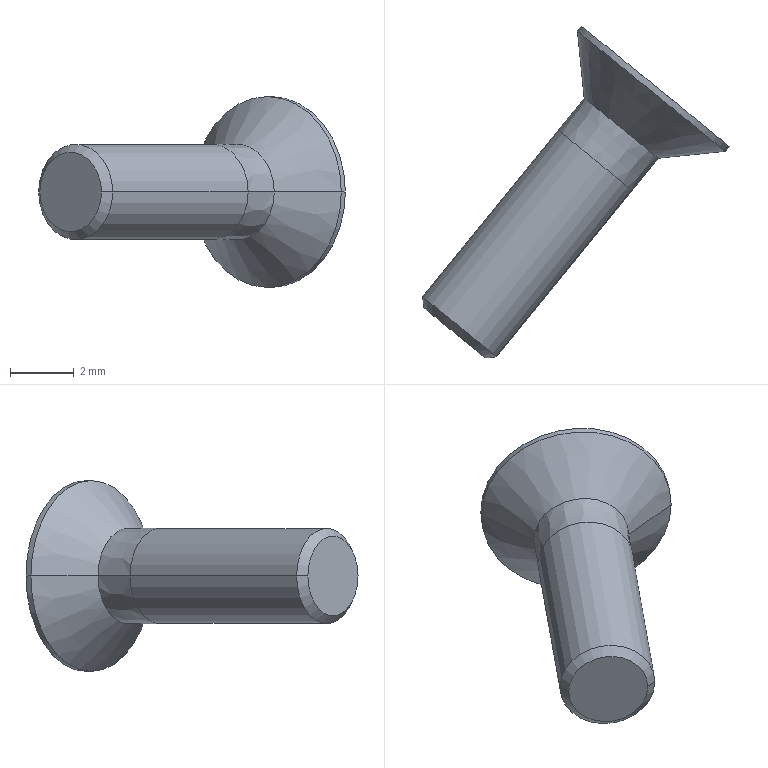Part | SolidWorks | features BaseBody 1 | 1 solid | 20 faces | box 9.643 x 10.44 x 6 mm | volume 84.627 mm3 | plane 10 | cone 6 | cylinder 4 | commonest cylinder face diameters 3 x2 6 x2
STEP:
#1=CARTESIAN_POINT('',(539.658,-134.219,294.945));
#2=VERTEX_POINT('',#1);
#3=CARTESIAN_POINT('',(537.331,-132.326,294.945));
#4=VERTEX_POINT('',#3);
#5=CARTESIAN_POINT('',(538.494,-133.273,294.945));
#6=DIRECTION('',(-0.6309,-0.7758,0.000000012));
#7=DIRECTION('',(0.7758,-0.6309,0.));
#8=AXIS2_PLACEMENT_3D('',#5,#6,#7);
#9=CIRCLE('',#8,1.5);
#10=EDGE_CURVE('',#2,#4,#9,.T.);
#11=ORIENTED_EDGE('',*,*,#10,.T.);
#12=CARTESIAN_POINT('',(533.072,-137.563,294.945));
#13=VERTEX_POINT('',#12);
#14=CARTESIAN_POINT('',(535.201,-134.945,294.945));
#15=DIRECTION('',(-0.6309,-0.7758,0.000000012));
#16=VECTOR('',#15,1000.);
#17=LINE('',#14,#16);
#18=EDGE_CURVE('',#4,#13,#17,.T.);
#19=ORIENTED_EDGE('',*,*,#18,.T.);
#20=CARTESIAN_POINT('',(535.399,-139.456,294.945));
#21=VERTEX_POINT('',#20);
#22=CARTESIAN_POINT('',(534.236,-138.51,294.945));
#23=DIRECTION('',(0.6309,0.7758,-0.000000012));
#24=DIRECTION('',(0.7758,-0.6309,0.));
#25=AXIS2_PLACEMENT_3D('',#22,#23,#24);
#26=CIRCLE('',#25,1.5);
#27=EDGE_CURVE('',#13,#21,#26,.T.);
#28=ORIENTED_EDGE('',*,*,#27,.T.);
#29=CARTESIAN_POINT('',(537.529,-136.838,294.945));
#30=DIRECTION('',(-0.6309,-0.7758,0.000000012));
#31=VECTOR('',#30,1000.);
#32=LINE('',#29,#31);
#33=EDGE_CURVE('',#2,#21,#32,.T.);
#34=ORIENTED_EDGE('',*,*,#33,.F.);
#35=EDGE_LOOP('',(#11,#19,#28,#34));
#36=FACE_OUTER_BOUND('',#35,.T.);
#37=CARTESIAN_POINT('',(536.365,-135.891,294.945));
#38=DIRECTION('',(-0.6309,-0.7758,0.000000012));
#39=DIRECTION('',(0.7758,-0.6309,0.));
#40=AXIS2_PLACEMENT_3D('',#37,#38,#39);
#41=CYLINDRICAL_SURFACE('',#40,1.5);
#42=ADVANCED_FACE('',(#36),#41,.T.);
#43=CARTESIAN_POINT('',(539.443,-132.368,296.435));
#44=VERTEX_POINT('',#43);
#45=CARTESIAN_POINT('',(538.151,-131.318,294.945));
#46=VERTEX_POINT('',#45);
#47=CARTESIAN_POINT('',(539.314,-132.264,294.945));
#48=DIRECTION('',(-0.6309,-0.7758,0.000000012));
#49=DIRECTION('',(0.7758,-0.6309,0.));
#50=AXIS2_PLACEMENT_3D('',#47,#48,#49);
#51=CIRCLE('',#50,1.5);
#52=EDGE_CURVE('',#44,#46,#51,.T.);
#53=ORIENTED_EDGE('',*,*,#52,.T.);
#54=CARTESIAN_POINT('',(537.331,-132.326,294.945));
#55=DIRECTION('',(-0.6311,-0.7757,0.000000012));
#56=VECTOR('',#55,1000.);
#57=LINE('',#54,#56);
#58=EDGE_CURVE('',#46,#4,#57,.T.);
#59=ORIENTED_EDGE('',*,*,#58,.T.);
#60=ORIENTED_EDGE('',*,*,#10,.F.);
#61=CARTESIAN_POINT('',(540.478,-133.21,294.945));
#62=VERTEX_POINT('',#61);
#63=CARTESIAN_POINT('',(539.658,-134.219,294.945));
#64=DIRECTION('',(-0.6307,-0.776,0.000000012));
#65=VECTOR('',#64,1000.);
#66=LINE('',#63,#65);
#67=EDGE_CURVE('',#62,#2,#66,.T.);
#68=ORIENTED_EDGE('',*,*,#67,.F.);
#69=CARTESIAN_POINT('',(539.315,-132.264,294.945));
#70=DIRECTION('',(-0.6309,-0.7758,0.000000012));
#71=DIRECTION('',(0.7758,-0.6309,0.));
#72=AXIS2_PLACEMENT_3D('',#69,#70,#71);
#73=CIRCLE('',#72,1.5);
#74=EDGE_CURVE('',#62,#44,#73,.T.);
#75=ORIENTED_EDGE('',*,*,#74,.T.);
#76=EDGE_LOOP('',(#53,#59,#60,#68,#75));
#77=FACE_OUTER_BOUND('',#76,.T.);
#78=CARTESIAN_POINT('',(538.494,-133.273,294.945));
#79=DIRECTION('',(-0.6309,-0.7758,0.000000012));
#80=DIRECTION('',(0.7758,-0.6309,0.));
#81=AXIS2_PLACEMENT_3D('',#78,#79,#80);
#82=CONICAL_SURFACE('',#81,1.5,0.00025);
#83=ADVANCED_FACE('',(#77),#82,.T.);
#84=CARTESIAN_POINT('',(533.108,-137.915,294.945));
#85=VERTEX_POINT('',#84);
#86=CARTESIAN_POINT('',(535.048,-139.492,294.945));
#87=VERTEX_POINT('',#86);
#88=CARTESIAN_POINT('',(534.078,-138.704,294.945));
#89=DIRECTION('',(0.6309,0.7758,-0.000000012));
#90=DIRECTION('',(-0.7758,0.6309,0.));
#91=AXIS2_PLACEMENT_3D('',#88,#89,#90);
#92=CIRCLE('',#91,1.25);
#93=EDGE_CURVE('',#85,#87,#92,.T.);
#94=ORIENTED_EDGE('',*,*,#93,.T.);
#95=CARTESIAN_POINT('',(535.399,-139.456,294.945));
#96=DIRECTION('',(0.9947,0.1025,-0.000000009));
#97=VECTOR('',#96,1000.);
#98=LINE('',#95,#97);
#99=EDGE_CURVE('',#87,#21,#98,.T.);
#100=ORIENTED_EDGE('',*,*,#99,.T.);
#101=ORIENTED_EDGE('',*,*,#27,.F.);
#102=CARTESIAN_POINT('',(533.072,-137.563,294.945));
#103=DIRECTION('',(-0.1025,0.9947,-0.000000009));
#104=VECTOR('',#103,1000.);
#105=LINE('',#102,#104);
#106=EDGE_CURVE('',#85,#13,#105,.T.);
#107=ORIENTED_EDGE('',*,*,#106,.F.);
#108=EDGE_LOOP('',(#94,#100,#101,#107));
#109=FACE_OUTER_BOUND('',#108,.T.);
#110=CARTESIAN_POINT('',(534.236,-138.51,294.945));
#111=DIRECTION('',(0.6309,0.7758,-0.000000012));
#112=DIRECTION('',(-0.7758,0.6309,0.));
#113=AXIS2_PLACEMENT_3D('',#110,#111,#112);
#114=CONICAL_SURFACE('',#113,1.5,0.7854);
#115=ADVANCED_FACE('',(#109),#114,.T.);
#116=CARTESIAN_POINT('',(540.478,-133.211,294.945));
#117=VERTEX_POINT('',#116);
#118=CARTESIAN_POINT('',(539.315,-132.264,294.945));
#119=DIRECTION('',(-0.6309,-0.7758,0.000000012));
#120=DIRECTION('',(-0.7758,0.6309,0.));
#121=AXIS2_PLACEMENT_3D('',#118,#119,#120);
#122=CIRCLE('',#121,1.5);
#123=EDGE_CURVE('',#117,#44,#122,.T.);
#124=ORIENTED_EDGE('',*,*,#123,.F.);
#125=CARTESIAN_POINT('',(542.588,-132.993,294.945));
#126=VERTEX_POINT('',#125);
#127=CARTESIAN_POINT('',(542.588,-132.993,294.945));
#128=DIRECTION('',(0.9947,0.1025,-0.000000009));
#129=VECTOR('',#128,1000.);
#130=LINE('',#127,#129);
#131=EDGE_CURVE('',#117,#126,#130,.T.);
#132=ORIENTED_EDGE('',*,*,#131,.T.);
#133=CARTESIAN_POINT('',(537.933,-129.208,294.945));
#134=VERTEX_POINT('',#133);
#135=CARTESIAN_POINT('',(540.261,-131.1,294.945));
#136=DIRECTION('',(-0.6309,-0.7758,0.000000012));
#137=DIRECTION('',(0.08545,-0.06949,0.9939));
#138=AXIS2_PLACEMENT_3D('',#135,#136,#137);
#139=CIRCLE('',#138,3.);
#140=EDGE_CURVE('',#126,#134,#139,.T.);
#141=ORIENTED_EDGE('',*,*,#140,.T.);
#142=CARTESIAN_POINT('',(537.933,-129.208,294.945));
#143=DIRECTION('',(-0.1025,0.9947,-0.000000009));
#144=VECTOR('',#143,1000.);
#145=LINE('',#142,#144);
#146=EDGE_CURVE('',#46,#134,#145,.T.);
#147=ORIENTED_EDGE('',*,*,#146,.F.);
#148=ORIENTED_EDGE('',*,*,#52,.F.);
#149=EDGE_LOOP('',(#124,#132,#141,#147,#148));
#150=FACE_OUTER_BOUND('',#149,.T.);
#151=CARTESIAN_POINT('',(540.261,-131.1,294.945));
#152=DIRECTION('',(0.6309,0.7758,-0.000000012));
#153=DIRECTION('',(-0.7758,0.6309,0.));
#154=AXIS2_PLACEMENT_3D('',#151,#152,#153);
#155=CONICAL_SURFACE('',#154,3.,0.7854);
#156=ADVANCED_FACE('',(#150),#155,.T.);
#157=CARTESIAN_POINT('',(542.715,-132.838,294.945));
#158=VERTEX_POINT('',#157);
#159=CARTESIAN_POINT('',(538.06,-129.053,294.945));
#160=VERTEX_POINT('',#159);
#161=CARTESIAN_POINT('',(540.387,-130.945,294.945));
#162=DIRECTION('',(-0.6309,-0.7758,0.000000012));
#163=DIRECTION('',(0.7758,-0.6309,0.));
#164=AXIS2_PLACEMENT_3D('',#161,#162,#163);
#165=CIRCLE('',#164,3.);
#166=EDGE_CURVE('',#158,#160,#165,.T.);
#167=ORIENTED_EDGE('',*,*,#166,.T.);
#168=CARTESIAN_POINT('',(537.997,-129.13,294.945));
#169=DIRECTION('',(-0.6309,-0.7758,0.000000012));
#170=VECTOR('',#169,1000.);
#171=LINE('',#168,#170);
#172=EDGE_CURVE('',#160,#134,#171,.T.);
#173=ORIENTED_EDGE('',*,*,#172,.T.);
#174=ORIENTED_EDGE('',*,*,#140,.F.);
#175=CARTESIAN_POINT('',(542.652,-132.916,294.945));
#176=DIRECTION('',(-0.6309,-0.7758,0.000000012));
#177=VECTOR('',#176,1000.);
#178=LINE('',#175,#177);
#179=EDGE_CURVE('',#158,#126,#178,.T.);
#180=ORIENTED_EDGE('',*,*,#179,.F.);
#181=EDGE_LOOP('',(#167,#173,#174,#180));
#182=FACE_OUTER_BOUND('',#181,.T.);
#183=CARTESIAN_POINT('',(540.324,-131.023,294.945));
#184=DIRECTION('',(-0.6309,-0.7758,0.000000012));
#185=DIRECTION('',(0.7758,-0.6309,0.));
#186=AXIS2_PLACEMENT_3D('',#183,#184,#185);
#187=CYLINDRICAL_SURFACE('',#186,3.);
#188=ADVANCED_FACE('',(#182),#187,.T.);
#189=ORIENTED_EDGE('',*,*,#18,.F.);
#190=CARTESIAN_POINT('',(538.494,-133.273,294.945));
#191=DIRECTION('',(-0.6309,-0.7758,0.000000012));
#192=DIRECTION('',(0.7758,-0.6309,0.));
#193=AXIS2_PLACEMENT_3D('',#190,#191,#192);
#194=CIRCLE('',#193,1.5);
#195=EDGE_CURVE('',#4,#2,#194,.T.);
#196=ORIENTED_EDGE('',*,*,#195,.T.);
#197=ORIENTED_EDGE('',*,*,#33,.T.);
#198=CARTESIAN_POINT('',(534.236,-138.51,294.945));
#199=DIRECTION('',(0.6309,0.7758,-0.000000012));
#200=DIRECTION('',(0.7758,-0.6309,0.));
#201=AXIS2_PLACEMENT_3D('',#198,#199,#200);
#202=CIRCLE('',#201,1.5);
#203=EDGE_CURVE('',#21,#13,#202,.T.);
#204=ORIENTED_EDGE('',*,*,#203,.T.);
#205=EDGE_LOOP('',(#189,#196,#197,#204));
#206=FACE_OUTER_BOUND('',#205,.T.);
#207=CARTESIAN_POINT('',(536.365,-135.891,294.945));
#208=DIRECTION('',(-0.6309,-0.7758,0.000000012));
#209=DIRECTION('',(0.7758,-0.6309,0.));
#210=AXIS2_PLACEMENT_3D('',#207,#208,#209);
#211=CYLINDRICAL_SURFACE('',#210,1.5);
#212=ADVANCED_FACE('',(#206),#211,.T.);
#213=ORIENTED_EDGE('',*,*,#58,.F.);
#214=CARTESIAN_POINT('',(539.186,-132.16,293.454));
#215=VERTEX_POINT('',#214);
#216=CARTESIAN_POINT('',(539.314,-132.264,294.945));
#217=DIRECTION('',(-0.6309,-0.7758,0.000000012));
#218=DIRECTION('',(0.7758,-0.6309,0.));
#219=AXIS2_PLACEMENT_3D('',#216,#217,#218);
#220=CIRCLE('',#219,1.5);
#221=EDGE_CURVE('',#46,#215,#220,.T.);
#222=ORIENTED_EDGE('',*,*,#221,.T.);
#223=CARTESIAN_POINT('',(539.315,-132.264,294.945));
#224=DIRECTION('',(-0.6309,-0.7758,0.000000012));
#225=DIRECTION('',(0.7758,-0.6309,0.));
#226=AXIS2_PLACEMENT_3D('',#223,#224,#225);
#227=CIRCLE('',#226,1.5);
#228=EDGE_CURVE('',#215,#62,#227,.T.);
#229=ORIENTED_EDGE('',*,*,#228,.T.);
#230=ORIENTED_EDGE('',*,*,#67,.T.);
#231=ORIENTED_EDGE('',*,*,#195,.F.);
#232=EDGE_LOOP('',(#213,#222,#229,#230,#231));
#233=FACE_OUTER_BOUND('',#232,.T.);
#234=CARTESIAN_POINT('',(538.494,-133.273,294.945));
#235=DIRECTION('',(-0.6309,-0.7758,0.000000012));
#236=DIRECTION('',(0.7758,-0.6309,0.));
#237=AXIS2_PLACEMENT_3D('',#234,#235,#236);
#238=CONICAL_SURFACE('',#237,1.5,0.00025);
#239=ADVANCED_FACE('',(#233),#238,.T.);
#240=ORIENTED_EDGE('',*,*,#99,.F.);
#241=CARTESIAN_POINT('',(534.078,-138.704,294.945));
#242=DIRECTION('',(0.6309,0.7758,-0.000000012));
#243=DIRECTION('',(-0.7758,0.6309,0.));
#244=AXIS2_PLACEMENT_3D('',#241,#242,#243);
#245=CIRCLE('',#244,1.25);
#246=EDGE_CURVE('',#87,#85,#245,.T.);
#247=ORIENTED_EDGE('',*,*,#246,.T.);
#248=ORIENTED_EDGE('',*,*,#106,.T.);
#249=ORIENTED_EDGE('',*,*,#203,.F.);
#250=EDGE_LOOP('',(#240,#247,#248,#249));
#251=FACE_OUTER_BOUND('',#250,.T.);
#252=CARTESIAN_POINT('',(534.236,-138.51,294.945));
#253=DIRECTION('',(0.6309,0.7758,-0.000000012));
#254=DIRECTION('',(-0.7758,0.6309,0.));
#255=AXIS2_PLACEMENT_3D('',#252,#253,#254);
#256=CONICAL_SURFACE('',#255,1.5,0.7854);
#257=ADVANCED_FACE('',(#251),#256,.T.);
#258=ORIENTED_EDGE('',*,*,#228,.F.);
#259=CARTESIAN_POINT('',(539.315,-132.264,294.945));
#260=DIRECTION('',(-0.6309,-0.7758,0.000000012));
#261=DIRECTION('',(-0.7758,0.6309,0.));
#262=AXIS2_PLACEMENT_3D('',#259,#260,#261);
#263=CIRCLE('',#262,1.5);
#264=EDGE_CURVE('',#215,#117,#263,.T.);
#265=ORIENTED_EDGE('',*,*,#264,.T.);
#266=ORIENTED_EDGE('',*,*,#123,.T.);
#267=ORIENTED_EDGE('',*,*,#74,.F.);
#268=EDGE_LOOP('',(#258,#265,#266,#267));
#269=FACE_OUTER_BOUND('',#268,.T.);
#270=CARTESIAN_POINT('',(539.379,-132.316,295.69));
#271=DIRECTION('',(-0.6309,-0.7758,0.000000012));
#272=DIRECTION('',(0.7758,-0.6309,0.));
#273=AXIS2_PLACEMENT_3D('',#270,#271,#272);
#274=PLANE('',#273);
#275=ADVANCED_FACE('',(#269),#274,.T.);
#276=ORIENTED_EDGE('',*,*,#93,.F.);
#277=ORIENTED_EDGE('',*,*,#246,.F.);
#278=EDGE_LOOP('',(#276,#277));
#279=FACE_OUTER_BOUND('',#278,.T.);
#280=CARTESIAN_POINT('',(534.131,-138.747,295.566));
#281=DIRECTION('',(-0.6309,-0.7758,0.000000012));
#282=DIRECTION('',(0.7758,-0.6309,0.));
#283=AXIS2_PLACEMENT_3D('',#280,#281,#282);
#284=PLANE('',#283);
#285=ADVANCED_FACE('',(#279),#284,.T.);
#286=ORIENTED_EDGE('',*,*,#131,.F.);
#287=ORIENTED_EDGE('',*,*,#264,.F.);
#288=ORIENTED_EDGE('',*,*,#221,.F.);
#289=ORIENTED_EDGE('',*,*,#146,.T.);
#290=CARTESIAN_POINT('',(540.261,-131.1,294.945));
#291=DIRECTION('',(-0.6309,-0.7758,0.000000012));
#292=DIRECTION('',(0.08545,-0.06949,0.9939));
#293=AXIS2_PLACEMENT_3D('',#290,#291,#292);
#294=CIRCLE('',#293,3.);
#295=EDGE_CURVE('',#134,#126,#294,.T.);
#296=ORIENTED_EDGE('',*,*,#295,.T.);
#297=EDGE_LOOP('',(#286,#287,#288,#289,#296));
#298=FACE_OUTER_BOUND('',#297,.T.);
#299=CARTESIAN_POINT('',(540.261,-131.1,294.945));
#300=DIRECTION('',(0.6309,0.7758,-0.000000012));
#301=DIRECTION('',(-0.7758,0.6309,0.));
#302=AXIS2_PLACEMENT_3D('',#299,#300,#301);
#303=CONICAL_SURFACE('',#302,3.,0.7854);
#304=ADVANCED_FACE('',(#298),#303,.T.);
#305=ORIENTED_EDGE('',*,*,#172,.F.);
#306=CARTESIAN_POINT('',(540.387,-130.945,294.945));
#307=DIRECTION('',(-0.6309,-0.7758,0.000000012));
#308=DIRECTION('',(0.7758,-0.6309,0.));
#309=AXIS2_PLACEMENT_3D('',#306,#307,#308);
#310=CIRCLE('',#309,3.);
#311=EDGE_CURVE('',#160,#158,#310,.T.);
#312=ORIENTED_EDGE('',*,*,#311,.T.);
#313=ORIENTED_EDGE('',*,*,#179,.T.);
#314=ORIENTED_EDGE('',*,*,#295,.F.);
#315=EDGE_LOOP('',(#305,#312,#313,#314));
#316=FACE_OUTER_BOUND('',#315,.T.);
#317=CARTESIAN_POINT('',(540.324,-131.023,294.945));
#318=DIRECTION('',(-0.6309,-0.7758,0.000000012));
#319=DIRECTION('',(0.7758,-0.6309,0.));
#320=AXIS2_PLACEMENT_3D('',#317,#318,#319);
#321=CYLINDRICAL_SURFACE('',#320,3.);
#322=ADVANCED_FACE('',(#316),#321,.T.);
#323=ORIENTED_EDGE('',*,*,#166,.F.);
#324=ORIENTED_EDGE('',*,*,#311,.F.);
#325=EDGE_LOOP('',(#323,#324));
#326=FACE_OUTER_BOUND('',#325,.T.);
#327=CARTESIAN_POINT('',(539.567,-130.278,294.481));
#328=VERTEX_POINT('',#327);
#329=CARTESIAN_POINT('',(540.288,-130.865,293.797));
#330=VERTEX_POINT('',#329);
#331=CARTESIAN_POINT('',(539.567,-130.278,294.481));
#332=DIRECTION('',(0.6251,-0.5083,-0.5923));
#333=VECTOR('',#332,1000.);
#334=LINE('',#331,#333);
#335=EDGE_CURVE('',#328,#330,#334,.T.);
#336=ORIENTED_EDGE('',*,*,#335,.T.);
#337=CARTESIAN_POINT('',(541.109,-131.532,294.261));
#338=VERTEX_POINT('',#337);
#339=CARTESIAN_POINT('',(540.288,-130.865,293.797));
#340=DIRECTION('',(0.7105,-0.5778,0.4016));
#341=VECTOR('',#340,1000.);
#342=LINE('',#339,#341);
#343=EDGE_CURVE('',#330,#338,#342,.T.);
#344=ORIENTED_EDGE('',*,*,#343,.T.);
#345=CARTESIAN_POINT('',(541.208,-131.613,295.408));
#346=VERTEX_POINT('',#345);
#347=CARTESIAN_POINT('',(541.109,-131.532,294.261));
#348=DIRECTION('',(0.08545,-0.06949,0.9939));
#349=VECTOR('',#348,1000.);
#350=LINE('',#347,#349);
#351=EDGE_CURVE('',#338,#346,#350,.T.);
#352=ORIENTED_EDGE('',*,*,#351,.T.);
#353=CARTESIAN_POINT('',(540.486,-131.026,296.092));
#354=VERTEX_POINT('',#353);
#355=CARTESIAN_POINT('',(541.208,-131.613,295.408));
#356=DIRECTION('',(-0.6251,0.5083,0.5923));
#357=VECTOR('',#356,1000.);
#358=LINE('',#355,#357);
#359=EDGE_CURVE('',#346,#354,#358,.T.);
#360=ORIENTED_EDGE('',*,*,#359,.T.);
#361=CARTESIAN_POINT('',(539.665,-130.358,295.629));
#362=VERTEX_POINT('',#361);
#363=CARTESIAN_POINT('',(540.486,-131.026,296.092));
#364=DIRECTION('',(-0.7105,0.5778,-0.4016));
#365=VECTOR('',#364,1000.);
#366=LINE('',#363,#365);
#367=EDGE_CURVE('',#354,#362,#366,.T.);
#368=ORIENTED_EDGE('',*,*,#367,.T.);
#369=CARTESIAN_POINT('',(539.665,-130.358,295.629));
#370=DIRECTION('',(-0.08545,0.06949,-0.9939));
#371=VECTOR('',#370,1000.);
#372=LINE('',#369,#371);
#373=EDGE_CURVE('',#362,#328,#372,.T.);
#374=ORIENTED_EDGE('',*,*,#373,.T.);
#375=EDGE_LOOP('',(#336,#344,#352,#360,#368,#374));
#376=FACE_BOUND('',#375,.T.);
#377=CARTESIAN_POINT('',(540.451,-130.997,295.69));
#378=DIRECTION('',(0.6309,0.7758,-0.000000012));
#379=DIRECTION('',(-0.7758,0.6309,0.));
#380=AXIS2_PLACEMENT_3D('',#377,#378,#379);
#381=PLANE('',#380);
#382=ADVANCED_FACE('',(#326,#376),#381,.T.);
#383=CARTESIAN_POINT('',(540.352,-132.463,294.261));
#384=VERTEX_POINT('',#383);
#385=CARTESIAN_POINT('',(541.109,-131.532,294.261));
#386=DIRECTION('',(-0.6309,-0.7758,0.000000012));
#387=VECTOR('',#386,1000.);
#388=LINE('',#385,#387);
#389=EDGE_CURVE('',#338,#384,#388,.T.);
#390=ORIENTED_EDGE('',*,*,#389,.F.);
#391=ORIENTED_EDGE('',*,*,#343,.F.);
#392=CARTESIAN_POINT('',(539.531,-131.796,293.797));
#393=VERTEX_POINT('',#392);
#394=CARTESIAN_POINT('',(539.531,-131.796,293.797));
#395=DIRECTION('',(0.6309,0.7758,-0.000000012));
#396=VECTOR('',#395,1000.);
#397=LINE('',#394,#396);
#398=EDGE_CURVE('',#393,#330,#397,.T.);
#399=ORIENTED_EDGE('',*,*,#398,.F.);
#400=CARTESIAN_POINT('',(540.352,-132.463,294.261));
#401=DIRECTION('',(-0.7105,0.5778,-0.4016));
#402=VECTOR('',#401,1000.);
#403=LINE('',#400,#402);
#404=EDGE_CURVE('',#384,#393,#403,.T.);
#405=ORIENTED_EDGE('',*,*,#404,.F.);
#406=EDGE_LOOP('',(#390,#391,#399,#405));
#407=FACE_OUTER_BOUND('',#406,.T.);
#408=CARTESIAN_POINT('',(541.109,-131.532,294.261));
#409=DIRECTION('',(0.3116,-0.2534,-0.9158));
#410=DIRECTION('',(-0.9467,0.,-0.3221));
#411=AXIS2_PLACEMENT_3D('',#408,#409,#410);
#412=PLANE('',#411);
#413=ADVANCED_FACE('',(#407),#412,.F.);
#414=ORIENTED_EDGE('',*,*,#398,.T.);
#415=ORIENTED_EDGE('',*,*,#335,.F.);
#416=CARTESIAN_POINT('',(538.81,-131.209,294.481));
#417=VERTEX_POINT('',#416);
#418=CARTESIAN_POINT('',(538.81,-131.209,294.481));
#419=DIRECTION('',(0.6309,0.7758,-0.000000012));
#420=VECTOR('',#419,1000.);
#421=LINE('',#418,#420);
#422=EDGE_CURVE('',#417,#328,#421,.T.);
#423=ORIENTED_EDGE('',*,*,#422,.F.);
#424=CARTESIAN_POINT('',(539.531,-131.796,293.797));
#425=DIRECTION('',(-0.6251,0.5083,0.5923));
#426=VECTOR('',#425,1000.);
#427=LINE('',#424,#426);
#428=EDGE_CURVE('',#393,#417,#427,.T.);
#429=ORIENTED_EDGE('',*,*,#428,.F.);
#430=EDGE_LOOP('',(#414,#415,#423,#429));
#431=FACE_OUTER_BOUND('',#430,.T.);
#432=CARTESIAN_POINT('',(540.288,-130.865,293.797));
#433=DIRECTION('',(-0.4596,0.3737,-0.8057));
#434=DIRECTION('',(-0.8686,0.,0.4955));
#435=AXIS2_PLACEMENT_3D('',#432,#433,#434);
#436=PLANE('',#435);
#437=ADVANCED_FACE('',(#431),#436,.F.);
#438=ORIENTED_EDGE('',*,*,#422,.T.);
#439=ORIENTED_EDGE('',*,*,#373,.F.);
#440=CARTESIAN_POINT('',(538.908,-131.289,295.629));
#441=VERTEX_POINT('',#440);
#442=CARTESIAN_POINT('',(539.665,-130.358,295.629));
#443=DIRECTION('',(0.6309,0.7758,0.));
#444=VECTOR('',#443,1000.);
#445=LINE('',#442,#444);
#446=EDGE_CURVE('',#441,#362,#445,.T.);
#447=ORIENTED_EDGE('',*,*,#446,.F.);
#448=CARTESIAN_POINT('',(538.81,-131.209,294.481));
#449=DIRECTION('',(0.08545,-0.06949,0.9939));
#450=VECTOR('',#449,1000.);
#451=LINE('',#448,#450);
#452=EDGE_CURVE('',#417,#441,#451,.T.);
#453=ORIENTED_EDGE('',*,*,#452,.F.);
#454=EDGE_LOOP('',(#438,#439,#447,#453));
#455=FACE_OUTER_BOUND('',#454,.T.);
#456=CARTESIAN_POINT('',(539.567,-130.278,294.481));
#457=DIRECTION('',(-0.7711,0.6271,0.1101));
#458=DIRECTION('',(-0.6309,-0.7758,0.));
#459=AXIS2_PLACEMENT_3D('',#456,#457,#458);
#460=PLANE('',#459);
#461=ADVANCED_FACE('',(#455),#460,.F.);
#462=ORIENTED_EDGE('',*,*,#446,.T.);
#463=ORIENTED_EDGE('',*,*,#367,.F.);
#464=CARTESIAN_POINT('',(539.729,-131.957,296.092));
#465=VERTEX_POINT('',#464);
#466=CARTESIAN_POINT('',(539.729,-131.957,296.092));
#467=DIRECTION('',(0.6309,0.7758,-0.000000012));
#468=VECTOR('',#467,1000.);
#469=LINE('',#466,#468);
#470=EDGE_CURVE('',#465,#354,#469,.T.);
#471=ORIENTED_EDGE('',*,*,#470,.F.);
#472=CARTESIAN_POINT('',(538.908,-131.289,295.629));
#473=DIRECTION('',(0.7105,-0.5778,0.4016));
#474=VECTOR('',#473,1000.);
#475=LINE('',#472,#474);
#476=EDGE_CURVE('',#441,#465,#475,.T.);
#477=ORIENTED_EDGE('',*,*,#476,.F.);
#478=EDGE_LOOP('',(#462,#463,#471,#477));
#479=FACE_OUTER_BOUND('',#478,.T.);
#480=CARTESIAN_POINT('',(539.665,-130.358,295.629));
#481=DIRECTION('',(-0.3116,0.2534,0.9158));
#482=DIRECTION('',(0.9467,0.,0.3221));
#483=AXIS2_PLACEMENT_3D('',#480,#481,#482);
#484=PLANE('',#483);
#485=ADVANCED_FACE('',(#479),#484,.F.);
#486=ORIENTED_EDGE('',*,*,#470,.T.);
#487=ORIENTED_EDGE('',*,*,#359,.F.);
#488=CARTESIAN_POINT('',(540.45,-132.544,295.408));
#489=VERTEX_POINT('',#488);
#490=CARTESIAN_POINT('',(540.45,-132.544,295.408));
#491=DIRECTION('',(0.6309,0.7758,-0.000000012));
#492=VECTOR('',#491,1000.);
#493=LINE('',#490,#492);
#494=EDGE_CURVE('',#489,#346,#493,.T.);
#495=ORIENTED_EDGE('',*,*,#494,.F.);
#496=CARTESIAN_POINT('',(539.729,-131.957,296.092));
#497=DIRECTION('',(0.6251,-0.5083,-0.5923));
#498=VECTOR('',#497,1000.);
#499=LINE('',#496,#498);
#500=EDGE_CURVE('',#465,#489,#499,.T.);
#501=ORIENTED_EDGE('',*,*,#500,.F.);
#502=EDGE_LOOP('',(#486,#487,#495,#501));
#503=FACE_OUTER_BOUND('',#502,.T.);
#504=CARTESIAN_POINT('',(540.486,-131.026,296.092));
#505=DIRECTION('',(0.4596,-0.3737,0.8057));
#506=DIRECTION('',(0.8686,0.,-0.4955));
#507=AXIS2_PLACEMENT_3D('',#504,#505,#506);
#508=PLANE('',#507);
#509=ADVANCED_FACE('',(#503),#508,.F.);
#510=ORIENTED_EDGE('',*,*,#494,.T.);
#511=ORIENTED_EDGE('',*,*,#351,.F.);
#512=ORIENTED_EDGE('',*,*,#389,.T.);
#513=CARTESIAN_POINT('',(540.45,-132.544,295.408));
#514=DIRECTION('',(-0.08545,0.06949,-0.9939));
#515=VECTOR('',#514,1000.);
#516=LINE('',#513,#515);
#517=EDGE_CURVE('',#489,#384,#516,.T.);
#518=ORIENTED_EDGE('',*,*,#517,.F.);
#519=EDGE_LOOP('',(#510,#511,#512,#518));
#520=FACE_OUTER_BOUND('',#519,.T.);
#521=CARTESIAN_POINT('',(541.208,-131.613,295.408));
#522=DIRECTION('',(0.7711,-0.6271,-0.1101));
#523=DIRECTION('',(0.6309,0.7758,0.));
#524=AXIS2_PLACEMENT_3D('',#521,#522,#523);
#525=PLANE('',#524);
#526=ADVANCED_FACE('',(#520),#525,.F.);
#527=ORIENTED_EDGE('',*,*,#476,.T.);
#528=ORIENTED_EDGE('',*,*,#500,.T.);
#529=ORIENTED_EDGE('',*,*,#517,.T.);
#530=ORIENTED_EDGE('',*,*,#404,.T.);
#531=ORIENTED_EDGE('',*,*,#428,.T.);
#532=ORIENTED_EDGE('',*,*,#452,.T.);
#533=EDGE_LOOP('',(#527,#528,#529,#530,#531,#532));
#534=FACE_OUTER_BOUND('',#533,.T.);
#535=CARTESIAN_POINT('',(539.63,-131.876,294.945));
#536=DIRECTION('',(0.6309,0.7758,-0.000000012));
#537=DIRECTION('',(-0.7758,0.6309,0.));
#538=AXIS2_PLACEMENT_3D('',#535,#536,#537);
#539=PLANE('',#538);
#540=ADVANCED_FACE('',(#534),#539,.T.);
#541=CLOSED_SHELL('',(#42,#83,#115,#156,#188,#212,#239,#257,#275,#285,#304,#322,#382,#413,#437,#461,#485,#509,#526,#540));
#542=MANIFOLD_SOLID_BREP('',#541);
#543=CARTESIAN_POINT('',(0.,0.,0.));
#544=DIRECTION('',(0.,0.,1.));
#545=DIRECTION('',(1.,0.,0.));
#546=AXIS2_PLACEMENT_3D('',#543,#544,#545);
#547=(LENGTH_UNIT()NAMED_UNIT(*)SI_UNIT(.MILLI.,.METRE.));
#548=UNCERTAINTY_MEASURE_WITH_UNIT(LENGTH_MEASURE(0.00001),#547,'','');
#549=(NAMED_UNIT(*)PLANE_ANGLE_UNIT()SI_UNIT($,.RADIAN.));
#550=(NAMED_UNIT(*)SI_UNIT($,.STERADIAN.)SOLID_ANGLE_UNIT());
#551=(GEOMETRIC_REPRESENTATION_CONTEXT(3)GLOBAL_UNCERTAINTY_ASSIGNED_CONTEXT((#548))GLOBAL_UNIT_ASSIGNED_CONTEXT((#547,#549,#550))REPRESENTATION_CONTEXT('',''));
#552=ADVANCED_BREP_SHAPE_REPRESENTATION('',(#542,#546),#551);